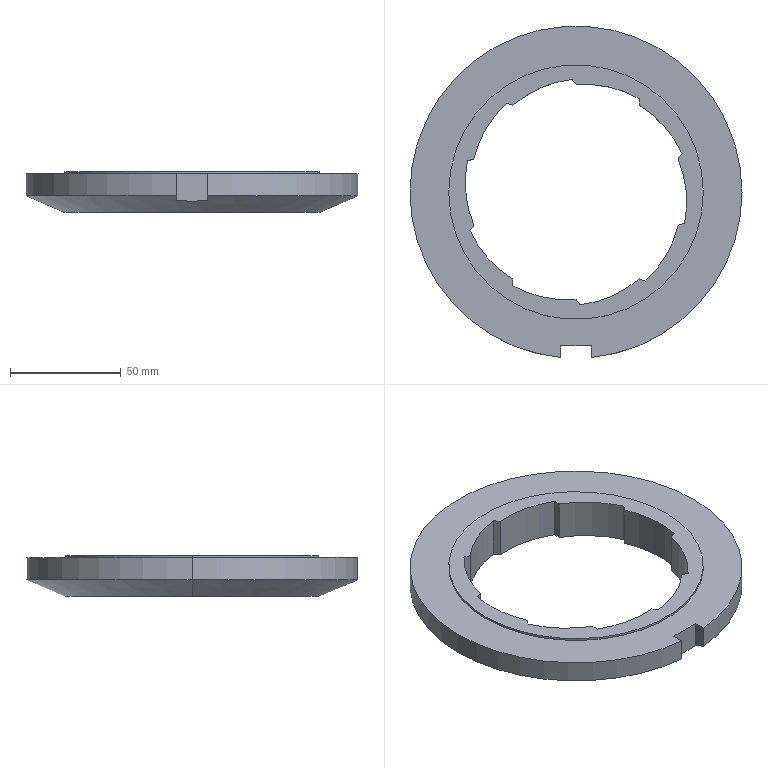Part | SolidWorks | features BaseBody 1, ICE 1 | 1 solid | 34 faces | box 150 x 149.673 x 18.5 mm | volume 146475 mm3 | cylinder 16 | plane 16 | cone 2 | commonest cylinder face diameters 100 x11 150 x3 115 x2
STEP:
#1=CARTESIAN_POINT('',(463.731,234.744,-733.193));
#2=VERTEX_POINT('',#1);
#3=CARTESIAN_POINT('',(578.731,234.744,-733.193));
#4=VERTEX_POINT('',#3);
#5=CARTESIAN_POINT('',(521.231,234.744,-733.193));
#6=DIRECTION('',(0.,0.,-1.));
#7=DIRECTION('',(-1.,0.,0.));
#8=AXIS2_PLACEMENT_3D('',#5,#6,#7);
#9=CIRCLE('',#8,57.5);
#10=EDGE_CURVE('',#2,#4,#9,.T.);
#11=ORIENTED_EDGE('',*,*,#10,.F.);
#12=CARTESIAN_POINT('',(446.231,234.744,-725.693));
#13=VERTEX_POINT('',#12);
#14=CARTESIAN_POINT('',(463.731,234.744,-733.193));
#15=DIRECTION('',(-0.9191,0.,0.3939));
#16=VECTOR('',#15,1000.);
#17=LINE('',#14,#16);
#18=EDGE_CURVE('',#2,#13,#17,.T.);
#19=ORIENTED_EDGE('',*,*,#18,.T.);
#20=CARTESIAN_POINT('',(596.231,234.744,-725.693));
#21=VERTEX_POINT('',#20);
#22=CARTESIAN_POINT('',(521.231,234.744,-725.693));
#23=DIRECTION('',(0.,0.,-1.));
#24=DIRECTION('',(-1.,0.,0.));
#25=AXIS2_PLACEMENT_3D('',#22,#23,#24);
#26=CIRCLE('',#25,75.);
#27=EDGE_CURVE('',#13,#21,#26,.T.);
#28=ORIENTED_EDGE('',*,*,#27,.T.);
#29=CARTESIAN_POINT('',(578.731,234.744,-733.193));
#30=DIRECTION('',(0.9191,0.,0.3939));
#31=VECTOR('',#30,1000.);
#32=LINE('',#29,#31);
#33=EDGE_CURVE('',#4,#21,#32,.T.);
#34=ORIENTED_EDGE('',*,*,#33,.F.);
#35=EDGE_LOOP('',(#11,#19,#28,#34));
#36=FACE_OUTER_BOUND('',#35,.T.);
#37=CARTESIAN_POINT('',(521.231,234.744,-733.193));
#38=DIRECTION('',(0.,0.,1.));
#39=DIRECTION('',(1.,0.,0.));
#40=AXIS2_PLACEMENT_3D('',#37,#38,#39);
#41=CONICAL_SURFACE('',#40,57.5,1.166);
#42=ADVANCED_FACE('',(#36),#41,.T.);
#43=CARTESIAN_POINT('',(578.731,234.744,-715.693));
#44=VERTEX_POINT('',#43);
#45=CARTESIAN_POINT('',(463.731,234.744,-715.693));
#46=VERTEX_POINT('',#45);
#47=CARTESIAN_POINT('',(521.231,234.744,-715.693));
#48=DIRECTION('',(0.,0.,1.));
#49=DIRECTION('',(1.,0.,0.));
#50=AXIS2_PLACEMENT_3D('',#47,#48,#49);
#51=CIRCLE('',#50,57.5);
#52=EDGE_CURVE('',#44,#46,#51,.T.);
#53=ORIENTED_EDGE('',*,*,#52,.T.);
#54=CARTESIAN_POINT('',(463.731,234.744,-714.693));
#55=VERTEX_POINT('',#54);
#56=CARTESIAN_POINT('',(463.731,234.744,-715.693));
#57=DIRECTION('',(0.,0.,1.));
#58=VECTOR('',#57,1000.);
#59=LINE('',#56,#58);
#60=EDGE_CURVE('',#46,#55,#59,.T.);
#61=ORIENTED_EDGE('',*,*,#60,.T.);
#62=CARTESIAN_POINT('',(578.731,234.744,-714.693));
#63=VERTEX_POINT('',#62);
#64=CARTESIAN_POINT('',(521.231,234.744,-714.693));
#65=DIRECTION('',(0.,0.,1.));
#66=DIRECTION('',(1.,0.,0.));
#67=AXIS2_PLACEMENT_3D('',#64,#65,#66);
#68=CIRCLE('',#67,57.5);
#69=EDGE_CURVE('',#63,#55,#68,.T.);
#70=ORIENTED_EDGE('',*,*,#69,.F.);
#71=CARTESIAN_POINT('',(578.731,234.744,-715.693));
#72=DIRECTION('',(0.,0.,1.));
#73=VECTOR('',#72,1000.);
#74=LINE('',#71,#73);
#75=EDGE_CURVE('',#44,#63,#74,.T.);
#76=ORIENTED_EDGE('',*,*,#75,.F.);
#77=EDGE_LOOP('',(#53,#61,#70,#76));
#78=FACE_OUTER_BOUND('',#77,.T.);
#79=CARTESIAN_POINT('',(521.231,234.744,-715.693));
#80=DIRECTION('',(0.,0.,1.));
#81=DIRECTION('',(1.,0.,0.));
#82=AXIS2_PLACEMENT_3D('',#79,#80,#81);
#83=CYLINDRICAL_SURFACE('',#82,57.5);
#84=ADVANCED_FACE('',(#78),#83,.T.);
#85=ORIENTED_EDGE('',*,*,#27,.F.);
#86=CARTESIAN_POINT('',(446.231,234.744,-715.693));
#87=VERTEX_POINT('',#86);
#88=CARTESIAN_POINT('',(446.231,234.744,-734.693));
#89=DIRECTION('',(0.,0.,1.));
#90=VECTOR('',#89,1000.);
#91=LINE('',#88,#90);
#92=EDGE_CURVE('',#13,#87,#91,.T.);
#93=ORIENTED_EDGE('',*,*,#92,.T.);
#94=CARTESIAN_POINT('',(596.231,234.744,-715.693));
#95=VERTEX_POINT('',#94);
#96=CARTESIAN_POINT('',(521.231,234.744,-715.693));
#97=DIRECTION('',(0.,0.,1.));
#98=DIRECTION('',(1.,0.,0.));
#99=AXIS2_PLACEMENT_3D('',#96,#97,#98);
#100=CIRCLE('',#99,75.);
#101=EDGE_CURVE('',#95,#87,#100,.T.);
#102=ORIENTED_EDGE('',*,*,#101,.F.);
#103=CARTESIAN_POINT('',(596.231,234.744,-734.693));
#104=DIRECTION('',(0.,0.,1.));
#105=VECTOR('',#104,1000.);
#106=LINE('',#103,#105);
#107=EDGE_CURVE('',#21,#95,#106,.T.);
#108=ORIENTED_EDGE('',*,*,#107,.F.);
#109=EDGE_LOOP('',(#85,#93,#102,#108));
#110=FACE_OUTER_BOUND('',#109,.T.);
#111=CARTESIAN_POINT('',(521.231,234.744,-734.693));
#112=DIRECTION('',(0.,0.,1.));
#113=DIRECTION('',(1.,0.,0.));
#114=AXIS2_PLACEMENT_3D('',#111,#112,#113);
#115=CYLINDRICAL_SURFACE('',#114,75.);
#116=ADVANCED_FACE('',(#110),#115,.T.);
#117=CARTESIAN_POINT('',(528.231,160.071,-725.693));
#118=VERTEX_POINT('',#117);
#119=CARTESIAN_POINT('',(521.231,234.744,-725.693));
#120=DIRECTION('',(0.,0.,-1.));
#121=DIRECTION('',(-1.,0.,0.));
#122=AXIS2_PLACEMENT_3D('',#119,#120,#121);
#123=CIRCLE('',#122,75.);
#124=EDGE_CURVE('',#21,#118,#123,.T.);
#125=ORIENTED_EDGE('',*,*,#124,.F.);
#126=ORIENTED_EDGE('',*,*,#107,.T.);
#127=CARTESIAN_POINT('',(528.231,160.071,-715.693));
#128=VERTEX_POINT('',#127);
#129=CARTESIAN_POINT('',(521.231,234.744,-715.693));
#130=DIRECTION('',(0.,0.,1.));
#131=DIRECTION('',(1.,0.,0.));
#132=AXIS2_PLACEMENT_3D('',#129,#130,#131);
#133=CIRCLE('',#132,75.);
#134=EDGE_CURVE('',#128,#95,#133,.T.);
#135=ORIENTED_EDGE('',*,*,#134,.F.);
#136=CARTESIAN_POINT('',(528.231,160.071,-734.693));
#137=DIRECTION('',(0.,0.,-1.));
#138=VECTOR('',#137,1000.);
#139=LINE('',#136,#138);
#140=EDGE_CURVE('',#128,#118,#139,.T.);
#141=ORIENTED_EDGE('',*,*,#140,.T.);
#142=EDGE_LOOP('',(#125,#126,#135,#141));
#143=FACE_OUTER_BOUND('',#142,.T.);
#144=CARTESIAN_POINT('',(521.231,234.744,-734.693));
#145=DIRECTION('',(0.,0.,1.));
#146=DIRECTION('',(1.,0.,0.));
#147=AXIS2_PLACEMENT_3D('',#144,#145,#146);
#148=CYLINDRICAL_SURFACE('',#147,75.);
#149=ADVANCED_FACE('',(#143),#148,.T.);
#150=CARTESIAN_POINT('',(471.242,239.027,-714.693));
#151=VERTEX_POINT('',#150);
#152=CARTESIAN_POINT('',(472.206,248.801,-714.693));
#153=VERTEX_POINT('',#152);
#154=CARTESIAN_POINT('',(521.242,239.027,-714.693));
#155=DIRECTION('',(0.,0.,-1.));
#156=DIRECTION('',(-1.,0.,0.));
#157=AXIS2_PLACEMENT_3D('',#154,#155,#156);
#158=CIRCLE('',#157,50.);
#159=EDGE_CURVE('',#151,#153,#158,.T.);
#160=ORIENTED_EDGE('',*,*,#159,.F.);
#161=CARTESIAN_POINT('',(471.242,239.027,-733.193));
#162=VERTEX_POINT('',#161);
#163=CARTESIAN_POINT('',(471.242,239.027,-506.693));
#164=DIRECTION('',(0.,0.,-1.));
#165=VECTOR('',#164,1000.);
#166=LINE('',#163,#165);
#167=EDGE_CURVE('',#151,#162,#166,.T.);
#168=ORIENTED_EDGE('',*,*,#167,.T.);
#169=CARTESIAN_POINT('',(472.206,248.801,-733.193));
#170=VERTEX_POINT('',#169);
#171=CARTESIAN_POINT('',(521.242,239.027,-733.193));
#172=DIRECTION('',(0.,0.,1.));
#173=DIRECTION('',(-1.,0.,0.));
#174=AXIS2_PLACEMENT_3D('',#171,#172,#173);
#175=CIRCLE('',#174,50.);
#176=EDGE_CURVE('',#170,#162,#175,.T.);
#177=ORIENTED_EDGE('',*,*,#176,.F.);
#178=CARTESIAN_POINT('',(472.206,248.801,-506.693));
#179=DIRECTION('',(0.,0.,-1.));
#180=VECTOR('',#179,1000.);
#181=LINE('',#178,#180);
#182=EDGE_CURVE('',#153,#170,#181,.T.);
#183=ORIENTED_EDGE('',*,*,#182,.F.);
#184=EDGE_LOOP('',(#160,#168,#177,#183));
#185=FACE_OUTER_BOUND('',#184,.T.);
#186=CARTESIAN_POINT('',(521.242,239.027,-506.693));
#187=DIRECTION('',(0.,0.,-1.));
#188=DIRECTION('',(-1.,0.,0.));
#189=AXIS2_PLACEMENT_3D('',#186,#187,#188);
#190=CYLINDRICAL_SURFACE('',#189,50.);
#191=ADVANCED_FACE('',(#185),#190,.F.);
#192=CARTESIAN_POINT('',(570.255,220.686,-733.193));
#193=VERTEX_POINT('',#192);
#194=CARTESIAN_POINT('',(567.357,249.731,-733.193));
#195=VERTEX_POINT('',#194);
#196=CARTESIAN_POINT('',(521.22,230.461,-733.193));
#197=DIRECTION('',(0.,0.,1.));
#198=DIRECTION('',(-1.,0.,0.));
#199=AXIS2_PLACEMENT_3D('',#196,#197,#198);
#200=CIRCLE('',#199,50.);
#201=EDGE_CURVE('',#193,#195,#200,.T.);
#202=ORIENTED_EDGE('',*,*,#201,.F.);
#203=CARTESIAN_POINT('',(570.255,220.686,-714.693));
#204=VERTEX_POINT('',#203);
#205=CARTESIAN_POINT('',(570.255,220.686,-506.693));
#206=DIRECTION('',(0.,0.,-1.));
#207=VECTOR('',#206,1000.);
#208=LINE('',#205,#207);
#209=EDGE_CURVE('',#204,#193,#208,.T.);
#210=ORIENTED_EDGE('',*,*,#209,.F.);
#211=CARTESIAN_POINT('',(567.357,249.731,-714.693));
#212=VERTEX_POINT('',#211);
#213=CARTESIAN_POINT('',(521.22,230.461,-714.693));
#214=DIRECTION('',(0.,0.,-1.));
#215=DIRECTION('',(-1.,0.,0.));
#216=AXIS2_PLACEMENT_3D('',#213,#214,#215);
#217=CIRCLE('',#216,50.);
#218=EDGE_CURVE('',#212,#204,#217,.T.);
#219=ORIENTED_EDGE('',*,*,#218,.F.);
#220=CARTESIAN_POINT('',(567.357,249.731,-506.693));
#221=DIRECTION('',(0.,0.,-1.));
#222=VECTOR('',#221,1000.);
#223=LINE('',#220,#222);
#224=EDGE_CURVE('',#212,#195,#223,.T.);
#225=ORIENTED_EDGE('',*,*,#224,.T.);
#226=EDGE_LOOP('',(#202,#210,#219,#225));
#227=FACE_OUTER_BOUND('',#226,.T.);
#228=CARTESIAN_POINT('',(521.22,230.461,-506.693));
#229=DIRECTION('',(0.,0.,-1.));
#230=DIRECTION('',(-1.,0.,0.));
#231=AXIS2_PLACEMENT_3D('',#228,#229,#230);
#232=CYLINDRICAL_SURFACE('',#231,50.);
#233=ADVANCED_FACE('',(#227),#232,.F.);
#234=CARTESIAN_POINT('',(489.832,274.933,-733.193));
#235=VERTEX_POINT('',#234);
#236=CARTESIAN_POINT('',(475.104,249.731,-733.193));
#237=VERTEX_POINT('',#236);
#238=CARTESIAN_POINT('',(523.757,238.203,-733.193));
#239=DIRECTION('',(0.,0.,1.));
#240=DIRECTION('',(-1.,0.,0.));
#241=AXIS2_PLACEMENT_3D('',#238,#239,#240);
#242=CIRCLE('',#241,50.);
#243=EDGE_CURVE('',#235,#237,#242,.T.);
#244=ORIENTED_EDGE('',*,*,#243,.F.);
#245=CARTESIAN_POINT('',(489.832,274.933,-714.693));
#246=VERTEX_POINT('',#245);
#247=CARTESIAN_POINT('',(489.832,274.933,-506.693));
#248=DIRECTION('',(0.,0.,-1.));
#249=VECTOR('',#248,1000.);
#250=LINE('',#247,#249);
#251=EDGE_CURVE('',#246,#235,#250,.T.);
#252=ORIENTED_EDGE('',*,*,#251,.F.);
#253=CARTESIAN_POINT('',(475.104,249.731,-714.693));
#254=VERTEX_POINT('',#253);
#255=CARTESIAN_POINT('',(523.757,238.203,-714.693));
#256=DIRECTION('',(0.,0.,-1.));
#257=DIRECTION('',(-1.,0.,0.));
#258=AXIS2_PLACEMENT_3D('',#255,#256,#257);
#259=CIRCLE('',#258,50.);
#260=EDGE_CURVE('',#254,#246,#259,.T.);
#261=ORIENTED_EDGE('',*,*,#260,.F.);
#262=CARTESIAN_POINT('',(475.104,249.731,-506.693));
#263=DIRECTION('',(0.,0.,-1.));
#264=VECTOR('',#263,1000.);
#265=LINE('',#262,#264);
#266=EDGE_CURVE('',#254,#237,#265,.T.);
#267=ORIENTED_EDGE('',*,*,#266,.T.);
#268=EDGE_LOOP('',(#244,#252,#261,#267));
#269=FACE_OUTER_BOUND('',#268,.T.);
#270=CARTESIAN_POINT('',(523.757,238.203,-506.693));
#271=DIRECTION('',(0.,0.,-1.));
#272=DIRECTION('',(-1.,0.,0.));
#273=AXIS2_PLACEMENT_3D('',#270,#271,#272);
#274=CYLINDRICAL_SURFACE('',#273,50.);
#275=ADVANCED_FACE('',(#269),#274,.F.);
#276=CARTESIAN_POINT('',(473.306,217.301,-733.193));
#277=VERTEX_POINT('',#276);
#278=CARTESIAN_POINT('',(492.723,195.507,-733.193));
#279=VERTEX_POINT('',#278);
#280=CARTESIAN_POINT('',(518.722,238.216,-733.193));
#281=DIRECTION('',(0.,0.,1.));
#282=DIRECTION('',(-1.,0.,0.));
#283=AXIS2_PLACEMENT_3D('',#280,#281,#282);
#284=CIRCLE('',#283,50.);
#285=EDGE_CURVE('',#277,#279,#284,.T.);
#286=ORIENTED_EDGE('',*,*,#285,.F.);
#287=CARTESIAN_POINT('',(473.306,217.301,-714.693));
#288=VERTEX_POINT('',#287);
#289=CARTESIAN_POINT('',(473.306,217.301,-506.693));
#290=DIRECTION('',(0.,0.,-1.));
#291=VECTOR('',#290,1000.);
#292=LINE('',#289,#291);
#293=EDGE_CURVE('',#288,#277,#292,.T.);
#294=ORIENTED_EDGE('',*,*,#293,.F.);
#295=CARTESIAN_POINT('',(492.723,195.507,-714.693));
#296=VERTEX_POINT('',#295);
#297=CARTESIAN_POINT('',(518.722,238.216,-714.693));
#298=DIRECTION('',(0.,0.,-1.));
#299=DIRECTION('',(-1.,0.,0.));
#300=AXIS2_PLACEMENT_3D('',#297,#298,#299);
#301=CIRCLE('',#300,50.);
#302=EDGE_CURVE('',#296,#288,#301,.T.);
#303=ORIENTED_EDGE('',*,*,#302,.F.);
#304=CARTESIAN_POINT('',(492.723,195.507,-506.693));
#305=DIRECTION('',(0.,0.,-1.));
#306=VECTOR('',#305,1000.);
#307=LINE('',#304,#306);
#308=EDGE_CURVE('',#296,#279,#307,.T.);
#309=ORIENTED_EDGE('',*,*,#308,.T.);
#310=EDGE_LOOP('',(#286,#294,#303,#309));
#311=FACE_OUTER_BOUND('',#310,.T.);
#312=CARTESIAN_POINT('',(518.722,238.216,-506.693));
#313=DIRECTION('',(0.,0.,-1.));
#314=DIRECTION('',(-1.,0.,0.));
#315=AXIS2_PLACEMENT_3D('',#312,#313,#314);
#316=CYLINDRICAL_SURFACE('',#315,50.);
#317=ADVANCED_FACE('',(#311),#316,.F.);
#318=CARTESIAN_POINT('',(523.011,183.775,-733.193));
#319=VERTEX_POINT('',#318);
#320=CARTESIAN_POINT('',(549.738,195.507,-733.193));
#321=VERTEX_POINT('',#320);
#322=CARTESIAN_POINT('',(517.154,233.431,-733.193));
#323=DIRECTION('',(0.,0.,1.));
#324=DIRECTION('',(-1.,0.,0.));
#325=AXIS2_PLACEMENT_3D('',#322,#323,#324);
#326=CIRCLE('',#325,50.);
#327=EDGE_CURVE('',#319,#321,#326,.T.);
#328=ORIENTED_EDGE('',*,*,#327,.F.);
#329=CARTESIAN_POINT('',(523.011,183.775,-714.693));
#330=VERTEX_POINT('',#329);
#331=CARTESIAN_POINT('',(523.011,183.775,-506.693));
#332=DIRECTION('',(0.,0.,-1.));
#333=VECTOR('',#332,1000.);
#334=LINE('',#331,#333);
#335=EDGE_CURVE('',#330,#319,#334,.T.);
#336=ORIENTED_EDGE('',*,*,#335,.F.);
#337=CARTESIAN_POINT('',(549.738,195.507,-714.693));
#338=VERTEX_POINT('',#337);
#339=CARTESIAN_POINT('',(517.154,233.431,-714.693));
#340=DIRECTION('',(0.,0.,-1.));
#341=DIRECTION('',(-1.,0.,0.));
#342=AXIS2_PLACEMENT_3D('',#339,#340,#341);
#343=CIRCLE('',#342,50.);
#344=EDGE_CURVE('',#338,#330,#343,.T.);
#345=ORIENTED_EDGE('',*,*,#344,.F.);
#346=CARTESIAN_POINT('',(549.738,195.507,-506.693));
#347=DIRECTION('',(0.,0.,-1.));
#348=VECTOR('',#347,1000.);
#349=LINE('',#346,#348);
#350=EDGE_CURVE('',#338,#321,#349,.T.);
#351=ORIENTED_EDGE('',*,*,#350,.T.);
#352=EDGE_LOOP('',(#328,#336,#345,#351));
#353=FACE_OUTER_BOUND('',#352,.T.);
#354=CARTESIAN_POINT('',(517.154,233.431,-506.693));
#355=DIRECTION('',(0.,0.,-1.));
#356=DIRECTION('',(-1.,0.,0.));
#357=AXIS2_PLACEMENT_3D('',#354,#355,#356);
#358=CYLINDRICAL_SURFACE('',#357,50.);
#359=ADVANCED_FACE('',(#353),#358,.F.);
#360=CARTESIAN_POINT('',(549.749,277.025,-733.193));
#361=VERTEX_POINT('',#360);
#362=CARTESIAN_POINT('',(521.231,283.244,-733.193));
#363=VERTEX_POINT('',#362);
#364=CARTESIAN_POINT('',(525.301,233.41,-733.193));
#365=DIRECTION('',(0.,0.,1.));
#366=DIRECTION('',(-1.,0.,0.));
#367=AXIS2_PLACEMENT_3D('',#364,#365,#366);
#368=CIRCLE('',#367,50.);
#369=EDGE_CURVE('',#361,#363,#368,.T.);
#370=ORIENTED_EDGE('',*,*,#369,.F.);
#371=CARTESIAN_POINT('',(549.749,277.025,-714.693));
#372=VERTEX_POINT('',#371);
#373=CARTESIAN_POINT('',(549.749,277.025,-506.693));
#374=DIRECTION('',(0.,0.,-1.));
#375=VECTOR('',#374,1000.);
#376=LINE('',#373,#375);
#377=EDGE_CURVE('',#372,#361,#376,.T.);
#378=ORIENTED_EDGE('',*,*,#377,.F.);
#379=CARTESIAN_POINT('',(521.231,283.244,-714.693));
#380=VERTEX_POINT('',#379);
#381=CARTESIAN_POINT('',(525.301,233.41,-714.693));
#382=DIRECTION('',(0.,0.,-1.));
#383=DIRECTION('',(-1.,0.,0.));
#384=AXIS2_PLACEMENT_3D('',#381,#382,#383);
#385=CIRCLE('',#384,50.);
#386=EDGE_CURVE('',#380,#372,#385,.T.);
#387=ORIENTED_EDGE('',*,*,#386,.F.);
#388=CARTESIAN_POINT('',(521.231,283.244,-506.693));
#389=DIRECTION('',(0.,0.,-1.));
#390=VECTOR('',#389,1000.);
#391=LINE('',#388,#390);
#392=EDGE_CURVE('',#380,#363,#391,.T.);
#393=ORIENTED_EDGE('',*,*,#392,.T.);
#394=EDGE_LOOP('',(#370,#378,#387,#393));
#395=FACE_OUTER_BOUND('',#394,.T.);
#396=CARTESIAN_POINT('',(525.301,233.41,-506.693));
#397=DIRECTION('',(0.,0.,-1.));
#398=DIRECTION('',(-1.,0.,0.));
#399=AXIS2_PLACEMENT_3D('',#396,#397,#398);
#400=CYLINDRICAL_SURFACE('',#399,50.);
#401=ADVANCED_FACE('',(#395),#400,.F.);
#402=ORIENTED_EDGE('',*,*,#335,.T.);
#403=CARTESIAN_POINT('',(521.231,186.244,-733.193));
#404=VERTEX_POINT('',#403);
#405=CARTESIAN_POINT('',(498.224,218.158,-733.193));
#406=DIRECTION('',(-0.5848,0.8112,0.));
#407=VECTOR('',#406,1000.);
#408=LINE('',#405,#407);
#409=EDGE_CURVE('',#319,#404,#408,.T.);
#410=ORIENTED_EDGE('',*,*,#409,.T.);
#411=CARTESIAN_POINT('',(521.231,186.244,-714.693));
#412=VERTEX_POINT('',#411);
#413=CARTESIAN_POINT('',(521.231,186.244,-506.693));
#414=DIRECTION('',(0.,0.,-1.));
#415=VECTOR('',#414,1000.);
#416=LINE('',#413,#415);
#417=EDGE_CURVE('',#412,#404,#416,.T.);
#418=ORIENTED_EDGE('',*,*,#417,.F.);
#419=CARTESIAN_POINT('',(498.224,218.158,-714.693));
#420=DIRECTION('',(0.5848,-0.8112,0.));
#421=VECTOR('',#420,1000.);
#422=LINE('',#419,#421);
#423=EDGE_CURVE('',#412,#330,#422,.T.);
#424=ORIENTED_EDGE('',*,*,#423,.T.);
#425=EDGE_LOOP('',(#402,#410,#418,#424));
#426=FACE_OUTER_BOUND('',#425,.T.);
#427=CARTESIAN_POINT('',(498.224,218.158,-506.693));
#428=DIRECTION('',(0.8112,0.5848,0.));
#429=DIRECTION('',(0.5848,-0.8112,0.));
#430=AXIS2_PLACEMENT_3D('',#427,#428,#429);
#431=PLANE('',#430);
#432=ADVANCED_FACE('',(#426),#431,.T.);
#433=ORIENTED_EDGE('',*,*,#209,.T.);
#434=CARTESIAN_POINT('',(567.357,219.757,-733.193));
#435=VERTEX_POINT('',#434);
#436=CARTESIAN_POINT('',(529.895,207.738,-733.193));
#437=DIRECTION('',(-0.9522,-0.3055,0.));
#438=VECTOR('',#437,1000.);
#439=LINE('',#436,#438);
#440=EDGE_CURVE('',#193,#435,#439,.T.);
#441=ORIENTED_EDGE('',*,*,#440,.T.);
#442=CARTESIAN_POINT('',(567.357,219.757,-714.693));
#443=VERTEX_POINT('',#442);
#444=CARTESIAN_POINT('',(567.357,219.757,-506.693));
#445=DIRECTION('',(0.,0.,-1.));
#446=VECTOR('',#445,1000.);
#447=LINE('',#444,#446);
#448=EDGE_CURVE('',#443,#435,#447,.T.);
#449=ORIENTED_EDGE('',*,*,#448,.F.);
#450=CARTESIAN_POINT('',(529.895,207.738,-714.693));
#451=DIRECTION('',(0.9522,0.3055,0.));
#452=VECTOR('',#451,1000.);
#453=LINE('',#450,#452);
#454=EDGE_CURVE('',#443,#204,#453,.T.);
#455=ORIENTED_EDGE('',*,*,#454,.T.);
#456=EDGE_LOOP('',(#433,#441,#449,#455));
#457=FACE_OUTER_BOUND('',#456,.T.);
#458=CARTESIAN_POINT('',(529.895,207.738,-506.693));
#459=DIRECTION('',(-0.3055,0.9522,0.));
#460=DIRECTION('',(0.9522,0.3055,0.));
#461=AXIS2_PLACEMENT_3D('',#458,#459,#460);
#462=PLANE('',#461);
#463=ADVANCED_FACE('',(#457),#462,.T.);
#464=ORIENTED_EDGE('',*,*,#377,.T.);
#465=CARTESIAN_POINT('',(549.738,273.981,-733.193));
#466=VERTEX_POINT('',#465);
#467=CARTESIAN_POINT('',(549.593,234.639,-733.193));
#468=DIRECTION('',(-0.003697,-1.,0.));
#469=VECTOR('',#468,1000.);
#470=LINE('',#467,#469);
#471=EDGE_CURVE('',#361,#466,#470,.T.);
#472=ORIENTED_EDGE('',*,*,#471,.T.);
#473=CARTESIAN_POINT('',(549.738,273.981,-714.693));
#474=VERTEX_POINT('',#473);
#475=CARTESIAN_POINT('',(549.738,273.981,-506.693));
#476=DIRECTION('',(0.,0.,-1.));
#477=VECTOR('',#476,1000.);
#478=LINE('',#475,#477);
#479=EDGE_CURVE('',#474,#466,#478,.T.);
#480=ORIENTED_EDGE('',*,*,#479,.F.);
#481=CARTESIAN_POINT('',(549.593,234.639,-714.693));
#482=DIRECTION('',(0.003697,1.,0.));
#483=VECTOR('',#482,1000.);
#484=LINE('',#481,#483);
#485=EDGE_CURVE('',#474,#372,#484,.T.);
#486=ORIENTED_EDGE('',*,*,#485,.T.);
#487=EDGE_LOOP('',(#464,#472,#480,#486));
#488=FACE_OUTER_BOUND('',#487,.T.);
#489=CARTESIAN_POINT('',(549.593,234.639,-506.693));
#490=DIRECTION('',(-1.,0.003697,0.));
#491=DIRECTION('',(0.003697,1.,0.));
#492=AXIS2_PLACEMENT_3D('',#489,#490,#491);
#493=PLANE('',#492);
#494=ADVANCED_FACE('',(#488),#493,.T.);
#495=ORIENTED_EDGE('',*,*,#251,.T.);
#496=CARTESIAN_POINT('',(492.723,273.981,-733.193));
#497=VERTEX_POINT('',#496);
#498=CARTESIAN_POINT('',(530.095,261.686,-733.193));
#499=DIRECTION('',(0.9499,-0.3125,0.));
#500=VECTOR('',#499,1000.);
#501=LINE('',#498,#500);
#502=EDGE_CURVE('',#235,#497,#501,.T.);
#503=ORIENTED_EDGE('',*,*,#502,.T.);
#504=CARTESIAN_POINT('',(492.723,273.981,-714.693));
#505=VERTEX_POINT('',#504);
#506=CARTESIAN_POINT('',(492.723,273.981,-506.693));
#507=DIRECTION('',(0.,0.,-1.));
#508=VECTOR('',#507,1000.);
#509=LINE('',#506,#508);
#510=EDGE_CURVE('',#505,#497,#509,.T.);
#511=ORIENTED_EDGE('',*,*,#510,.F.);
#512=CARTESIAN_POINT('',(530.095,261.686,-714.693));
#513=DIRECTION('',(-0.9499,0.3125,0.));
#514=VECTOR('',#513,1000.);
#515=LINE('',#512,#514);
#516=EDGE_CURVE('',#505,#246,#515,.T.);
#517=ORIENTED_EDGE('',*,*,#516,.T.);
#518=EDGE_LOOP('',(#495,#503,#511,#517));
#519=FACE_OUTER_BOUND('',#518,.T.);
#520=CARTESIAN_POINT('',(530.095,261.686,-506.693));
#521=DIRECTION('',(-0.3125,-0.9499,0.));
#522=DIRECTION('',(-0.9499,0.3125,0.));
#523=AXIS2_PLACEMENT_3D('',#520,#521,#522);
#524=PLANE('',#523);
#525=ADVANCED_FACE('',(#519),#524,.T.);
#526=ORIENTED_EDGE('',*,*,#293,.T.);
#527=CARTESIAN_POINT('',(475.104,219.757,-733.193));
#528=VERTEX_POINT('',#527);
#529=CARTESIAN_POINT('',(498.347,251.5,-733.193));
#530=DIRECTION('',(0.5908,0.8068,0.));
#531=VECTOR('',#530,1000.);
#532=LINE('',#529,#531);
#533=EDGE_CURVE('',#277,#528,#532,.T.);
#534=ORIENTED_EDGE('',*,*,#533,.T.);
#535=CARTESIAN_POINT('',(475.104,219.757,-714.693));
#536=VERTEX_POINT('',#535);
#537=CARTESIAN_POINT('',(475.104,219.757,-506.693));
#538=DIRECTION('',(0.,0.,-1.));
#539=VECTOR('',#538,1000.);
#540=LINE('',#537,#539);
#541=EDGE_CURVE('',#536,#528,#540,.T.);
#542=ORIENTED_EDGE('',*,*,#541,.F.);
#543=CARTESIAN_POINT('',(498.347,251.5,-714.693));
#544=DIRECTION('',(-0.5908,-0.8068,0.));
#545=VECTOR('',#544,1000.);
#546=LINE('',#543,#545);
#547=EDGE_CURVE('',#536,#288,#546,.T.);
#548=ORIENTED_EDGE('',*,*,#547,.T.);
#549=EDGE_LOOP('',(#526,#534,#542,#548));
#550=FACE_OUTER_BOUND('',#549,.T.);
#551=CARTESIAN_POINT('',(498.347,251.5,-506.693));
#552=DIRECTION('',(0.8068,-0.5908,0.));
#553=DIRECTION('',(-0.5908,-0.8068,0.));
#554=AXIS2_PLACEMENT_3D('',#551,#552,#553);
#555=PLANE('',#554);
#556=ADVANCED_FACE('',(#550),#555,.T.);
#557=CARTESIAN_POINT('',(492.712,192.463,-733.193));
#558=VERTEX_POINT('',#557);
#559=CARTESIAN_POINT('',(517.16,236.078,-733.193));
#560=DIRECTION('',(0.,0.,1.));
#561=DIRECTION('',(-1.,0.,0.));
#562=AXIS2_PLACEMENT_3D('',#559,#560,#561);
#563=CIRCLE('',#562,50.);
#564=EDGE_CURVE('',#558,#404,#563,.T.);
#565=ORIENTED_EDGE('',*,*,#564,.F.);
#566=CARTESIAN_POINT('',(492.712,192.463,-714.693));
#567=VERTEX_POINT('',#566);
#568=CARTESIAN_POINT('',(492.712,192.463,-506.693));
#569=DIRECTION('',(0.,0.,-1.));
#570=VECTOR('',#569,1000.);
#571=LINE('',#568,#570);
#572=EDGE_CURVE('',#567,#558,#571,.T.);
#573=ORIENTED_EDGE('',*,*,#572,.F.);
#574=CARTESIAN_POINT('',(517.16,236.078,-714.693));
#575=DIRECTION('',(0.,0.,-1.));
#576=DIRECTION('',(-1.,0.,0.));
#577=AXIS2_PLACEMENT_3D('',#574,#575,#576);
#578=CIRCLE('',#577,50.);
#579=EDGE_CURVE('',#412,#567,#578,.T.);
#580=ORIENTED_EDGE('',*,*,#579,.F.);
#581=ORIENTED_EDGE('',*,*,#417,.T.);
#582=EDGE_LOOP('',(#565,#573,#580,#581));
#583=FACE_OUTER_BOUND('',#582,.T.);
#584=CARTESIAN_POINT('',(517.16,236.078,-506.693));
#585=DIRECTION('',(0.,0.,-1.));
#586=DIRECTION('',(-1.,0.,0.));
#587=AXIS2_PLACEMENT_3D('',#584,#585,#586);
#588=CYLINDRICAL_SURFACE('',#587,50.);
#589=ADVANCED_FACE('',(#583),#588,.F.);
#590=CARTESIAN_POINT('',(552.629,194.555,-733.193));
#591=VERTEX_POINT('',#590);
#592=CARTESIAN_POINT('',(518.704,231.285,-733.193));
#593=DIRECTION('',(0.,0.,1.));
#594=DIRECTION('',(-1.,0.,0.));
#595=AXIS2_PLACEMENT_3D('',#592,#593,#594);
#596=CIRCLE('',#595,50.);
#597=EDGE_CURVE('',#591,#435,#596,.T.);
#598=ORIENTED_EDGE('',*,*,#597,.F.);
#599=CARTESIAN_POINT('',(552.629,194.555,-714.693));
#600=VERTEX_POINT('',#599);
#601=CARTESIAN_POINT('',(552.629,194.555,-506.693));
#602=DIRECTION('',(0.,0.,-1.));
#603=VECTOR('',#602,1000.);
#604=LINE('',#601,#603);
#605=EDGE_CURVE('',#600,#591,#604,.T.);
#606=ORIENTED_EDGE('',*,*,#605,.F.);
#607=CARTESIAN_POINT('',(518.704,231.285,-714.693));
#608=DIRECTION('',(0.,0.,-1.));
#609=DIRECTION('',(-1.,0.,0.));
#610=AXIS2_PLACEMENT_3D('',#607,#608,#609);
#611=CIRCLE('',#610,50.);
#612=EDGE_CURVE('',#443,#600,#611,.T.);
#613=ORIENTED_EDGE('',*,*,#612,.F.);
#614=ORIENTED_EDGE('',*,*,#448,.T.);
#615=EDGE_LOOP('',(#598,#606,#613,#614));
#616=FACE_OUTER_BOUND('',#615,.T.);
#617=CARTESIAN_POINT('',(518.704,231.285,-506.693));
#618=DIRECTION('',(0.,0.,-1.));
#619=DIRECTION('',(-1.,0.,0.));
#620=AXIS2_PLACEMENT_3D('',#617,#618,#619);
#621=CYLINDRICAL_SURFACE('',#620,50.);
#622=ADVANCED_FACE('',(#616),#621,.F.);
#623=CARTESIAN_POINT('',(569.155,252.187,-733.193));
#624=VERTEX_POINT('',#623);
#625=CARTESIAN_POINT('',(523.739,231.272,-733.193));
#626=DIRECTION('',(0.,0.,1.));
#627=DIRECTION('',(-1.,0.,0.));
#628=AXIS2_PLACEMENT_3D('',#625,#626,#627);
#629=CIRCLE('',#628,50.);
#630=EDGE_CURVE('',#624,#466,#629,.T.);
#631=ORIENTED_EDGE('',*,*,#630,.F.);
#632=CARTESIAN_POINT('',(569.155,252.187,-714.693));
#633=VERTEX_POINT('',#632);
#634=CARTESIAN_POINT('',(569.155,252.187,-506.693));
#635=DIRECTION('',(0.,0.,-1.));
#636=VECTOR('',#635,1000.);
#637=LINE('',#634,#636);
#638=EDGE_CURVE('',#633,#624,#637,.T.);
#639=ORIENTED_EDGE('',*,*,#638,.F.);
#640=CARTESIAN_POINT('',(523.739,231.272,-714.693));
#641=DIRECTION('',(0.,0.,-1.));
#642=DIRECTION('',(-1.,0.,0.));
#643=AXIS2_PLACEMENT_3D('',#640,#641,#642);
#644=CIRCLE('',#643,50.);
#645=EDGE_CURVE('',#474,#633,#644,.T.);
#646=ORIENTED_EDGE('',*,*,#645,.F.);
#647=ORIENTED_EDGE('',*,*,#479,.T.);
#648=EDGE_LOOP('',(#631,#639,#646,#647));
#649=FACE_OUTER_BOUND('',#648,.T.);
#650=CARTESIAN_POINT('',(523.739,231.272,-506.693));
#651=DIRECTION('',(0.,0.,-1.));
#652=DIRECTION('',(-1.,0.,0.));
#653=AXIS2_PLACEMENT_3D('',#650,#651,#652);
#654=CYLINDRICAL_SURFACE('',#653,50.);
#655=ADVANCED_FACE('',(#649),#654,.F.);
#656=CARTESIAN_POINT('',(519.451,285.713,-733.193));
#657=VERTEX_POINT('',#656);
#658=CARTESIAN_POINT('',(525.308,236.057,-733.193));
#659=DIRECTION('',(0.,0.,1.));
#660=DIRECTION('',(-1.,0.,0.));
#661=AXIS2_PLACEMENT_3D('',#658,#659,#660);
#662=CIRCLE('',#661,50.);
#663=EDGE_CURVE('',#657,#497,#662,.T.);
#664=ORIENTED_EDGE('',*,*,#663,.F.);
#665=CARTESIAN_POINT('',(519.451,285.713,-714.693));
#666=VERTEX_POINT('',#665);
#667=CARTESIAN_POINT('',(519.451,285.713,-506.693));
#668=DIRECTION('',(0.,0.,-1.));
#669=VECTOR('',#668,1000.);
#670=LINE('',#667,#669);
#671=EDGE_CURVE('',#666,#657,#670,.T.);
#672=ORIENTED_EDGE('',*,*,#671,.F.);
#673=CARTESIAN_POINT('',(525.308,236.057,-714.693));
#674=DIRECTION('',(0.,0.,-1.));
#675=DIRECTION('',(-1.,0.,0.));
#676=AXIS2_PLACEMENT_3D('',#673,#674,#675);
#677=CIRCLE('',#676,50.);
#678=EDGE_CURVE('',#505,#666,#677,.T.);
#679=ORIENTED_EDGE('',*,*,#678,.F.);
#680=ORIENTED_EDGE('',*,*,#510,.T.);
#681=EDGE_LOOP('',(#664,#672,#679,#680));
#682=FACE_OUTER_BOUND('',#681,.T.);
#683=CARTESIAN_POINT('',(525.308,236.057,-506.693));
#684=DIRECTION('',(0.,0.,-1.));
#685=DIRECTION('',(-1.,0.,0.));
#686=AXIS2_PLACEMENT_3D('',#683,#684,#685);
#687=CYLINDRICAL_SURFACE('',#686,50.);
#688=ADVANCED_FACE('',(#682),#687,.F.);
#689=ORIENTED_EDGE('',*,*,#167,.F.);
#690=CARTESIAN_POINT('',(521.242,239.027,-714.693));
#691=DIRECTION('',(0.,0.,-1.));
#692=DIRECTION('',(-1.,0.,0.));
#693=AXIS2_PLACEMENT_3D('',#690,#691,#692);
#694=CIRCLE('',#693,50.);
#695=EDGE_CURVE('',#536,#151,#694,.T.);
#696=ORIENTED_EDGE('',*,*,#695,.F.);
#697=ORIENTED_EDGE('',*,*,#541,.T.);
#698=CARTESIAN_POINT('',(521.242,239.027,-733.193));
#699=DIRECTION('',(0.,0.,1.));
#700=DIRECTION('',(-1.,0.,0.));
#701=AXIS2_PLACEMENT_3D('',#698,#699,#700);
#702=CIRCLE('',#701,50.);
#703=EDGE_CURVE('',#162,#528,#702,.T.);
#704=ORIENTED_EDGE('',*,*,#703,.F.);
#705=EDGE_LOOP('',(#689,#696,#697,#704));
#706=FACE_OUTER_BOUND('',#705,.T.);
#707=CARTESIAN_POINT('',(521.242,239.027,-506.693));
#708=DIRECTION('',(0.,0.,-1.));
#709=DIRECTION('',(-1.,0.,0.));
#710=AXIS2_PLACEMENT_3D('',#707,#708,#709);
#711=CYLINDRICAL_SURFACE('',#710,50.);
#712=ADVANCED_FACE('',(#706),#711,.F.);
#713=ORIENTED_EDGE('',*,*,#605,.T.);
#714=CARTESIAN_POINT('',(512.367,207.802,-733.193));
#715=DIRECTION('',(-0.9499,0.3125,0.));
#716=VECTOR('',#715,1000.);
#717=LINE('',#714,#716);
#718=EDGE_CURVE('',#591,#321,#717,.T.);
#719=ORIENTED_EDGE('',*,*,#718,.T.);
#720=ORIENTED_EDGE('',*,*,#350,.F.);
#721=CARTESIAN_POINT('',(512.367,207.802,-714.693));
#722=DIRECTION('',(0.9499,-0.3125,0.));
#723=VECTOR('',#722,1000.);
#724=LINE('',#721,#723);
#725=EDGE_CURVE('',#338,#600,#724,.T.);
#726=ORIENTED_EDGE('',*,*,#725,.T.);
#727=EDGE_LOOP('',(#713,#719,#720,#726));
#728=FACE_OUTER_BOUND('',#727,.T.);
#729=CARTESIAN_POINT('',(512.367,207.802,-506.693));
#730=DIRECTION('',(0.3125,0.9499,0.));
#731=DIRECTION('',(0.9499,-0.3125,0.));
#732=AXIS2_PLACEMENT_3D('',#729,#730,#731);
#733=PLANE('',#732);
#734=ADVANCED_FACE('',(#728),#733,.T.);
#735=ORIENTED_EDGE('',*,*,#638,.T.);
#736=CARTESIAN_POINT('',(544.114,217.988,-733.193));
#737=DIRECTION('',(-0.5908,-0.8068,0.));
#738=VECTOR('',#737,1000.);
#739=LINE('',#736,#738);
#740=EDGE_CURVE('',#624,#195,#739,.T.);
#741=ORIENTED_EDGE('',*,*,#740,.T.);
#742=ORIENTED_EDGE('',*,*,#224,.F.);
#743=CARTESIAN_POINT('',(544.114,217.988,-714.693));
#744=DIRECTION('',(0.5908,0.8068,0.));
#745=VECTOR('',#744,1000.);
#746=LINE('',#743,#745);
#747=EDGE_CURVE('',#212,#633,#746,.T.);
#748=ORIENTED_EDGE('',*,*,#747,.T.);
#749=EDGE_LOOP('',(#735,#741,#742,#748));
#750=FACE_OUTER_BOUND('',#749,.T.);
#751=CARTESIAN_POINT('',(544.114,217.988,-506.693));
#752=DIRECTION('',(-0.8068,0.5908,0.));
#753=DIRECTION('',(0.5908,0.8068,0.));
#754=AXIS2_PLACEMENT_3D('',#751,#752,#753);
#755=PLANE('',#754);
#756=ADVANCED_FACE('',(#750),#755,.T.);
#757=ORIENTED_EDGE('',*,*,#182,.T.);
#758=CARTESIAN_POINT('',(512.566,261.75,-733.193));
#759=DIRECTION('',(0.9522,0.3055,0.));
#760=VECTOR('',#759,1000.);
#761=LINE('',#758,#760);
#762=EDGE_CURVE('',#170,#237,#761,.T.);
#763=ORIENTED_EDGE('',*,*,#762,.T.);
#764=ORIENTED_EDGE('',*,*,#266,.F.);
#765=CARTESIAN_POINT('',(512.566,261.75,-714.693));
#766=DIRECTION('',(-0.9522,-0.3055,0.));
#767=VECTOR('',#766,1000.);
#768=LINE('',#765,#767);
#769=EDGE_CURVE('',#254,#153,#768,.T.);
#770=ORIENTED_EDGE('',*,*,#769,.T.);
#771=EDGE_LOOP('',(#757,#763,#764,#770));
#772=FACE_OUTER_BOUND('',#771,.T.);
#773=CARTESIAN_POINT('',(512.566,261.75,-506.693));
#774=DIRECTION('',(0.3055,-0.9522,0.));
#775=DIRECTION('',(-0.9522,-0.3055,0.));
#776=AXIS2_PLACEMENT_3D('',#773,#774,#775);
#777=PLANE('',#776);
#778=ADVANCED_FACE('',(#772),#777,.T.);
#779=ORIENTED_EDGE('',*,*,#572,.T.);
#780=CARTESIAN_POINT('',(492.869,234.849,-733.193));
#781=DIRECTION('',(0.003697,1.,0.));
#782=VECTOR('',#781,1000.);
#783=LINE('',#780,#782);
#784=EDGE_CURVE('',#558,#279,#783,.T.);
#785=ORIENTED_EDGE('',*,*,#784,.T.);
#786=ORIENTED_EDGE('',*,*,#308,.F.);
#787=CARTESIAN_POINT('',(492.869,234.849,-714.693));
#788=DIRECTION('',(-0.003697,-1.,0.));
#789=VECTOR('',#788,1000.);
#790=LINE('',#787,#789);
#791=EDGE_CURVE('',#296,#567,#790,.T.);
#792=ORIENTED_EDGE('',*,*,#791,.T.);
#793=EDGE_LOOP('',(#779,#785,#786,#792));
#794=FACE_OUTER_BOUND('',#793,.T.);
#795=CARTESIAN_POINT('',(492.869,234.849,-506.693));
#796=DIRECTION('',(1.,-0.003697,0.));
#797=DIRECTION('',(-0.003697,-1.,0.));
#798=AXIS2_PLACEMENT_3D('',#795,#796,#797);
#799=PLANE('',#798);
#800=ADVANCED_FACE('',(#794),#799,.T.);
#801=ORIENTED_EDGE('',*,*,#671,.T.);
#802=CARTESIAN_POINT('',(544.238,251.33,-733.193));
#803=DIRECTION('',(0.5848,-0.8112,0.));
#804=VECTOR('',#803,1000.);
#805=LINE('',#802,#804);
#806=EDGE_CURVE('',#657,#363,#805,.T.);
#807=ORIENTED_EDGE('',*,*,#806,.T.);
#808=ORIENTED_EDGE('',*,*,#392,.F.);
#809=CARTESIAN_POINT('',(544.238,251.33,-714.693));
#810=DIRECTION('',(-0.5848,0.8112,0.));
#811=VECTOR('',#810,1000.);
#812=LINE('',#809,#811);
#813=EDGE_CURVE('',#380,#666,#812,.T.);
#814=ORIENTED_EDGE('',*,*,#813,.T.);
#815=EDGE_LOOP('',(#801,#807,#808,#814));
#816=FACE_OUTER_BOUND('',#815,.T.);
#817=CARTESIAN_POINT('',(544.238,251.33,-506.693));
#818=DIRECTION('',(-0.8112,-0.5848,0.));
#819=DIRECTION('',(-0.5848,0.8112,0.));
#820=AXIS2_PLACEMENT_3D('',#817,#818,#819);
#821=PLANE('',#820);
#822=ADVANCED_FACE('',(#816),#821,.T.);
#823=ORIENTED_EDGE('',*,*,#725,.F.);
#824=ORIENTED_EDGE('',*,*,#344,.T.);
#825=ORIENTED_EDGE('',*,*,#423,.F.);
#826=ORIENTED_EDGE('',*,*,#579,.T.);
#827=ORIENTED_EDGE('',*,*,#791,.F.);
#828=ORIENTED_EDGE('',*,*,#302,.T.);
#829=ORIENTED_EDGE('',*,*,#547,.F.);
#830=ORIENTED_EDGE('',*,*,#695,.T.);
#831=ORIENTED_EDGE('',*,*,#159,.T.);
#832=ORIENTED_EDGE('',*,*,#769,.F.);
#833=ORIENTED_EDGE('',*,*,#260,.T.);
#834=ORIENTED_EDGE('',*,*,#516,.F.);
#835=ORIENTED_EDGE('',*,*,#678,.T.);
#836=ORIENTED_EDGE('',*,*,#813,.F.);
#837=ORIENTED_EDGE('',*,*,#386,.T.);
#838=ORIENTED_EDGE('',*,*,#485,.F.);
#839=ORIENTED_EDGE('',*,*,#645,.T.);
#840=ORIENTED_EDGE('',*,*,#747,.F.);
#841=ORIENTED_EDGE('',*,*,#218,.T.);
#842=ORIENTED_EDGE('',*,*,#454,.F.);
#843=ORIENTED_EDGE('',*,*,#612,.T.);
#844=EDGE_LOOP('',(#823,#824,#825,#826,#827,#828,#829,#830,#831,#832,#833,#834,#835,#836,#837,#838,#839,#840,#841,#842,#843));
#845=FACE_BOUND('',#844,.T.);
#846=ORIENTED_EDGE('',*,*,#69,.T.);
#847=CARTESIAN_POINT('',(521.231,234.744,-714.693));
#848=DIRECTION('',(0.,0.,1.));
#849=DIRECTION('',(1.,0.,0.));
#850=AXIS2_PLACEMENT_3D('',#847,#848,#849);
#851=CIRCLE('',#850,57.5);
#852=EDGE_CURVE('',#55,#63,#851,.T.);
#853=ORIENTED_EDGE('',*,*,#852,.T.);
#854=EDGE_LOOP('',(#846,#853));
#855=FACE_OUTER_BOUND('',#854,.T.);
#856=CARTESIAN_POINT('',(521.231,234.744,-714.693));
#857=DIRECTION('',(0.,0.,-1.));
#858=DIRECTION('',(-1.,0.,0.));
#859=AXIS2_PLACEMENT_3D('',#856,#857,#858);
#860=PLANE('',#859);
#861=ADVANCED_FACE('',(#845,#855),#860,.F.);
#862=ORIENTED_EDGE('',*,*,#92,.F.);
#863=CARTESIAN_POINT('',(514.231,160.071,-725.693));
#864=VERTEX_POINT('',#863);
#865=CARTESIAN_POINT('',(521.231,234.744,-725.693));
#866=DIRECTION('',(0.,0.,-1.));
#867=DIRECTION('',(-1.,0.,0.));
#868=AXIS2_PLACEMENT_3D('',#865,#866,#867);
#869=CIRCLE('',#868,75.);
#870=EDGE_CURVE('',#864,#13,#869,.T.);
#871=ORIENTED_EDGE('',*,*,#870,.F.);
#872=CARTESIAN_POINT('',(514.231,160.071,-715.693));
#873=VERTEX_POINT('',#872);
#874=CARTESIAN_POINT('',(514.231,160.071,-734.693));
#875=DIRECTION('',(0.,0.,1.));
#876=VECTOR('',#875,1000.);
#877=LINE('',#874,#876);
#878=EDGE_CURVE('',#864,#873,#877,.T.);
#879=ORIENTED_EDGE('',*,*,#878,.T.);
#880=CARTESIAN_POINT('',(521.231,234.744,-715.693));
#881=DIRECTION('',(0.,0.,1.));
#882=DIRECTION('',(1.,0.,0.));
#883=AXIS2_PLACEMENT_3D('',#880,#881,#882);
#884=CIRCLE('',#883,75.);
#885=EDGE_CURVE('',#87,#873,#884,.T.);
#886=ORIENTED_EDGE('',*,*,#885,.F.);
#887=EDGE_LOOP('',(#862,#871,#879,#886));
#888=FACE_OUTER_BOUND('',#887,.T.);
#889=CARTESIAN_POINT('',(521.231,234.744,-734.693));
#890=DIRECTION('',(0.,0.,1.));
#891=DIRECTION('',(1.,0.,0.));
#892=AXIS2_PLACEMENT_3D('',#889,#890,#891);
#893=CYLINDRICAL_SURFACE('',#892,75.);
#894=ADVANCED_FACE('',(#888),#893,.T.);
#895=CARTESIAN_POINT('',(528.231,165.244,-715.693));
#896=VERTEX_POINT('',#895);
#897=CARTESIAN_POINT('',(528.231,234.744,-715.693));
#898=DIRECTION('',(0.,1.,0.));
#899=VECTOR('',#898,1000.);
#900=LINE('',#897,#899);
#901=EDGE_CURVE('',#128,#896,#900,.T.);
#902=ORIENTED_EDGE('',*,*,#901,.F.);
#903=ORIENTED_EDGE('',*,*,#134,.T.);
#904=ORIENTED_EDGE('',*,*,#101,.T.);
#905=ORIENTED_EDGE('',*,*,#885,.T.);
#906=CARTESIAN_POINT('',(514.231,165.244,-715.693));
#907=VERTEX_POINT('',#906);
#908=CARTESIAN_POINT('',(514.231,234.744,-715.693));
#909=DIRECTION('',(0.,-1.,0.));
#910=VECTOR('',#909,1000.);
#911=LINE('',#908,#910);
#912=EDGE_CURVE('',#907,#873,#911,.T.);
#913=ORIENTED_EDGE('',*,*,#912,.F.);
#914=CARTESIAN_POINT('',(521.231,165.244,-715.693));
#915=DIRECTION('',(-1.,0.,0.));
#916=VECTOR('',#915,1000.);
#917=LINE('',#914,#916);
#918=EDGE_CURVE('',#896,#907,#917,.T.);
#919=ORIENTED_EDGE('',*,*,#918,.F.);
#920=EDGE_LOOP('',(#902,#903,#904,#905,#913,#919));
#921=FACE_OUTER_BOUND('',#920,.T.);
#922=ORIENTED_EDGE('',*,*,#52,.F.);
#923=CARTESIAN_POINT('',(521.231,234.744,-715.693));
#924=DIRECTION('',(0.,0.,1.));
#925=DIRECTION('',(1.,0.,0.));
#926=AXIS2_PLACEMENT_3D('',#923,#924,#925);
#927=CIRCLE('',#926,57.5);
#928=EDGE_CURVE('',#46,#44,#927,.T.);
#929=ORIENTED_EDGE('',*,*,#928,.F.);
#930=EDGE_LOOP('',(#922,#929));
#931=FACE_BOUND('',#930,.T.);
#932=CARTESIAN_POINT('',(521.231,234.744,-715.693));
#933=DIRECTION('',(0.,0.,1.));
#934=DIRECTION('',(1.,0.,0.));
#935=AXIS2_PLACEMENT_3D('',#932,#933,#934);
#936=PLANE('',#935);
#937=ADVANCED_FACE('',(#921,#931),#936,.T.);
#938=ORIENTED_EDGE('',*,*,#60,.F.);
#939=ORIENTED_EDGE('',*,*,#928,.T.);
#940=ORIENTED_EDGE('',*,*,#75,.T.);
#941=ORIENTED_EDGE('',*,*,#852,.F.);
#942=EDGE_LOOP('',(#938,#939,#940,#941));
#943=FACE_OUTER_BOUND('',#942,.T.);
#944=CARTESIAN_POINT('',(521.231,234.744,-715.693));
#945=DIRECTION('',(0.,0.,1.));
#946=DIRECTION('',(1.,0.,0.));
#947=AXIS2_PLACEMENT_3D('',#944,#945,#946);
#948=CYLINDRICAL_SURFACE('',#947,57.5);
#949=ADVANCED_FACE('',(#943),#948,.T.);
#950=ORIENTED_EDGE('',*,*,#18,.F.);
#951=CARTESIAN_POINT('',(521.231,234.744,-733.193));
#952=DIRECTION('',(0.,0.,-1.));
#953=DIRECTION('',(-1.,0.,0.));
#954=AXIS2_PLACEMENT_3D('',#951,#952,#953);
#955=CIRCLE('',#954,57.5);
#956=EDGE_CURVE('',#4,#2,#955,.T.);
#957=ORIENTED_EDGE('',*,*,#956,.F.);
#958=ORIENTED_EDGE('',*,*,#33,.T.);
#959=ORIENTED_EDGE('',*,*,#124,.T.);
#960=CARTESIAN_POINT('',(528.231,165.244,-727.899));
#961=VERTEX_POINT('',#960);
#962=CARTESIAN_POINT('',(528.231,165.244,-727.899));
#963=CARTESIAN_POINT('',(528.231,163.52,-727.164));
#964=CARTESIAN_POINT('',(528.231,161.795,-726.429));
#965=CARTESIAN_POINT('',(528.231,160.071,-725.693));
#966=B_SPLINE_CURVE_WITH_KNOTS('',3,(#962,#963,#964,#965),.UNSPECIFIED.,.F.,.F.,(4,4),(0.01344,0.01907),.UNSPECIFIED.);
#967=EDGE_CURVE('',#961,#118,#966,.T.);
#968=ORIENTED_EDGE('',*,*,#967,.F.);
#969=CARTESIAN_POINT('',(514.231,165.244,-727.899));
#970=VERTEX_POINT('',#969);
#971=CARTESIAN_POINT('',(514.231,165.244,-727.899));
#972=CARTESIAN_POINT('',(516.558,165.244,-727.999));
#973=CARTESIAN_POINT('',(518.888,165.244,-728.05));
#974=CARTESIAN_POINT('',(523.556,165.244,-728.05));
#975=CARTESIAN_POINT('',(525.895,165.244,-728.));
#976=CARTESIAN_POINT('',(528.231,165.244,-727.899));
#977=B_SPLINE_CURVE_WITH_KNOTS('',3,(#971,#972,#973,#974,#975,#976),.UNSPECIFIED.,.F.,.F.,(4,2,4),(0.01928,0.02627,0.03325),.UNSPECIFIED.);
#978=EDGE_CURVE('',#970,#961,#977,.T.);
#979=ORIENTED_EDGE('',*,*,#978,.F.);
#980=CARTESIAN_POINT('',(514.231,160.071,-725.693));
#981=CARTESIAN_POINT('',(514.231,161.795,-726.429));
#982=CARTESIAN_POINT('',(514.231,163.52,-727.164));
#983=CARTESIAN_POINT('',(514.231,165.244,-727.899));
#984=B_SPLINE_CURVE_WITH_KNOTS('',3,(#980,#981,#982,#983),.UNSPECIFIED.,.F.,.F.,(4,4),(0.0164,0.02203),.UNSPECIFIED.);
#985=EDGE_CURVE('',#864,#970,#984,.T.);
#986=ORIENTED_EDGE('',*,*,#985,.F.);
#987=ORIENTED_EDGE('',*,*,#870,.T.);
#988=EDGE_LOOP('',(#950,#957,#958,#959,#968,#979,#986,#987));
#989=FACE_OUTER_BOUND('',#988,.T.);
#990=CARTESIAN_POINT('',(521.231,234.744,-733.193));
#991=DIRECTION('',(0.,0.,1.));
#992=DIRECTION('',(1.,0.,0.));
#993=AXIS2_PLACEMENT_3D('',#990,#991,#992);
#994=CONICAL_SURFACE('',#993,57.5,1.166);
#995=ADVANCED_FACE('',(#989),#994,.T.);
#996=ORIENTED_EDGE('',*,*,#918,.T.);
#997=CARTESIAN_POINT('',(514.231,165.244,-805.693));
#998=DIRECTION('',(0.,0.,1.));
#999=VECTOR('',#998,1000.);
#1000=LINE('',#997,#999);
#1001=EDGE_CURVE('',#970,#907,#1000,.T.);
#1002=ORIENTED_EDGE('',*,*,#1001,.F.);
#1003=ORIENTED_EDGE('',*,*,#978,.T.);
#1004=CARTESIAN_POINT('',(528.231,165.244,-805.693));
#1005=DIRECTION('',(0.,0.,1.));
#1006=VECTOR('',#1005,1000.);
#1007=LINE('',#1004,#1006);
#1008=EDGE_CURVE('',#961,#896,#1007,.T.);
#1009=ORIENTED_EDGE('',*,*,#1008,.T.);
#1010=EDGE_LOOP('',(#996,#1002,#1003,#1009));
#1011=FACE_OUTER_BOUND('',#1010,.T.);
#1012=CARTESIAN_POINT('',(528.231,165.244,-805.693));
#1013=DIRECTION('',(0.,1.,0.));
#1014=DIRECTION('',(0.,0.,-1.));
#1015=AXIS2_PLACEMENT_3D('',#1012,#1013,#1014);
#1016=PLANE('',#1015);
#1017=ADVANCED_FACE('',(#1011),#1016,.F.);
#1018=ORIENTED_EDGE('',*,*,#901,.T.);
#1019=ORIENTED_EDGE('',*,*,#1008,.F.);
#1020=ORIENTED_EDGE('',*,*,#967,.T.);
#1021=ORIENTED_EDGE('',*,*,#140,.F.);
#1022=EDGE_LOOP('',(#1018,#1019,#1020,#1021));
#1023=FACE_OUTER_BOUND('',#1022,.T.);
#1024=CARTESIAN_POINT('',(528.231,147.41,-805.693));
#1025=DIRECTION('',(1.,0.,0.));
#1026=DIRECTION('',(0.,-1.,0.));
#1027=AXIS2_PLACEMENT_3D('',#1024,#1025,#1026);
#1028=PLANE('',#1027);
#1029=ADVANCED_FACE('',(#1023),#1028,.F.);
#1030=ORIENTED_EDGE('',*,*,#912,.T.);
#1031=ORIENTED_EDGE('',*,*,#878,.F.);
#1032=ORIENTED_EDGE('',*,*,#985,.T.);
#1033=ORIENTED_EDGE('',*,*,#1001,.T.);
#1034=EDGE_LOOP('',(#1030,#1031,#1032,#1033));
#1035=FACE_OUTER_BOUND('',#1034,.T.);
#1036=CARTESIAN_POINT('',(514.231,165.244,-805.693));
#1037=DIRECTION('',(-1.,0.,0.));
#1038=DIRECTION('',(0.,1.,0.));
#1039=AXIS2_PLACEMENT_3D('',#1036,#1037,#1038);
#1040=PLANE('',#1039);
#1041=ADVANCED_FACE('',(#1035),#1040,.F.);
#1042=ORIENTED_EDGE('',*,*,#956,.T.);
#1043=ORIENTED_EDGE('',*,*,#10,.T.);
#1044=EDGE_LOOP('',(#1042,#1043));
#1045=FACE_OUTER_BOUND('',#1044,.T.);
#1046=ORIENTED_EDGE('',*,*,#201,.T.);
#1047=ORIENTED_EDGE('',*,*,#740,.F.);
#1048=ORIENTED_EDGE('',*,*,#630,.T.);
#1049=ORIENTED_EDGE('',*,*,#471,.F.);
#1050=ORIENTED_EDGE('',*,*,#369,.T.);
#1051=ORIENTED_EDGE('',*,*,#806,.F.);
#1052=ORIENTED_EDGE('',*,*,#663,.T.);
#1053=ORIENTED_EDGE('',*,*,#502,.F.);
#1054=ORIENTED_EDGE('',*,*,#243,.T.);
#1055=ORIENTED_EDGE('',*,*,#762,.F.);
#1056=ORIENTED_EDGE('',*,*,#176,.T.);
#1057=ORIENTED_EDGE('',*,*,#703,.T.);
#1058=ORIENTED_EDGE('',*,*,#533,.F.);
#1059=ORIENTED_EDGE('',*,*,#285,.T.);
#1060=ORIENTED_EDGE('',*,*,#784,.F.);
#1061=ORIENTED_EDGE('',*,*,#564,.T.);
#1062=ORIENTED_EDGE('',*,*,#409,.F.);
#1063=ORIENTED_EDGE('',*,*,#327,.T.);
#1064=ORIENTED_EDGE('',*,*,#718,.F.);
#1065=ORIENTED_EDGE('',*,*,#597,.T.);
#1066=ORIENTED_EDGE('',*,*,#440,.F.);
#1067=EDGE_LOOP('',(#1046,#1047,#1048,#1049,#1050,#1051,#1052,#1053,#1054,#1055,#1056,#1057,#1058,#1059,#1060,#1061,#1062,#1063,#1064,#1065,#1066));
#1068=FACE_BOUND('',#1067,.T.);
#1069=CARTESIAN_POINT('',(521.231,234.744,-733.193));
#1070=DIRECTION('',(0.,0.,-1.));
#1071=DIRECTION('',(-1.,0.,0.));
#1072=AXIS2_PLACEMENT_3D('',#1069,#1070,#1071);
#1073=PLANE('',#1072);
#1074=ADVANCED_FACE('',(#1045,#1068),#1073,.T.);
#1075=CLOSED_SHELL('',(#42,#84,#116,#149,#191,#233,#275,#317,#359,#401,#432,#463,#494,#525,#556,#589,#622,#655,#688,#712,#734,#756,#778,#800,#822,#861,#894,#937,#949,#995,#1017,#1029,#1041,#1074));
#1076=MANIFOLD_SOLID_BREP('',#1075);
#1077=CARTESIAN_POINT('',(0.,0.,0.));
#1078=DIRECTION('',(0.,0.,1.));
#1079=DIRECTION('',(1.,0.,0.));
#1080=AXIS2_PLACEMENT_3D('',#1077,#1078,#1079);
#1081=(LENGTH_UNIT()NAMED_UNIT(*)SI_UNIT(.MILLI.,.METRE.));
#1082=UNCERTAINTY_MEASURE_WITH_UNIT(LENGTH_MEASURE(0.00001),#1081,'','');
#1083=(NAMED_UNIT(*)PLANE_ANGLE_UNIT()SI_UNIT($,.RADIAN.));
#1084=(NAMED_UNIT(*)SI_UNIT($,.STERADIAN.)SOLID_ANGLE_UNIT());
#1085=(GEOMETRIC_REPRESENTATION_CONTEXT(3)GLOBAL_UNCERTAINTY_ASSIGNED_CONTEXT((#1082))GLOBAL_UNIT_ASSIGNED_CONTEXT((#1081,#1083,#1084))REPRESENTATION_CONTEXT('',''));
#1086=ADVANCED_BREP_SHAPE_REPRESENTATION('',(#1076,#1080),#1085);